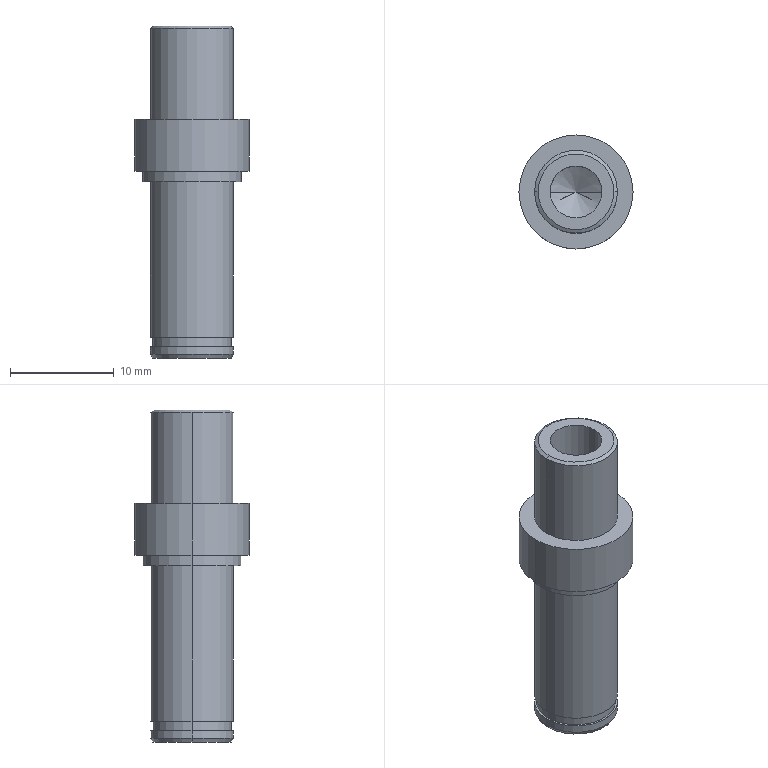Part | STEP file | FBDS-CS-032 | 1 solid | 27 faces | box 11 x 11 x 32 mm | volume 1542 mm3 | cylinder 14 | plane 7 | cone 6 | commonest cylinder face diameters 8 x6 5 x2 7.6 x2 9.5 x2 11 x2
STEP:
#1=CARTESIAN_POINT('',(3.654,0.,32.));
#2=VERTEX_POINT('',#1);
#3=CARTESIAN_POINT('',(-3.654,0.,32.));
#4=VERTEX_POINT('',#3);
#5=CARTESIAN_POINT('',(0.,0.,32.));
#6=DIRECTION('',(0.,0.,1.));
#7=DIRECTION('',(1.,0.,0.));
#8=AXIS2_PLACEMENT_3D('',#5,#6,#7);
#9=CIRCLE('',#8,3.654);
#10=EDGE_CURVE('',#2,#4,#9,.T.);
#11=ORIENTED_EDGE('',*,*,#10,.F.);
#12=CARTESIAN_POINT('',(4.,0.,31.8));
#13=VERTEX_POINT('',#12);
#14=CARTESIAN_POINT('',(3.654,0.,32.));
#15=DIRECTION('',(0.866,0.,-0.5));
#16=VECTOR('',#15,1000.);
#17=LINE('',#14,#16);
#18=EDGE_CURVE('',#2,#13,#17,.T.);
#19=ORIENTED_EDGE('',*,*,#18,.T.);
#20=CARTESIAN_POINT('',(-4.,0.,31.8));
#21=VERTEX_POINT('',#20);
#22=CARTESIAN_POINT('',(0.,0.,31.8));
#23=DIRECTION('',(0.,0.,-1.));
#24=DIRECTION('',(1.,0.,0.));
#25=AXIS2_PLACEMENT_3D('',#22,#23,#24);
#26=CIRCLE('',#25,4.);
#27=EDGE_CURVE('',#21,#13,#26,.T.);
#28=ORIENTED_EDGE('',*,*,#27,.F.);
#29=CARTESIAN_POINT('',(-3.654,0.,32.));
#30=DIRECTION('',(-0.866,0.,-0.5));
#31=VECTOR('',#30,1000.);
#32=LINE('',#29,#31);
#33=EDGE_CURVE('',#4,#21,#32,.T.);
#34=ORIENTED_EDGE('',*,*,#33,.F.);
#35=EDGE_LOOP('',(#11,#19,#28,#34));
#36=FACE_OUTER_BOUND('',#35,.T.);
#37=CARTESIAN_POINT('',(0.,0.,32.));
#38=DIRECTION('',(0.,0.,-1.));
#39=DIRECTION('',(-1.,0.,0.));
#40=AXIS2_PLACEMENT_3D('',#37,#38,#39);
#41=CONICAL_SURFACE('',#40,3.654,1.047);
#42=ADVANCED_FACE('',(#36),#41,.T.);
#43=CARTESIAN_POINT('',(-3.8,0.,0.));
#44=VERTEX_POINT('',#43);
#45=CARTESIAN_POINT('',(3.8,0.,0.));
#46=VERTEX_POINT('',#45);
#47=CARTESIAN_POINT('',(0.,0.,0.));
#48=DIRECTION('',(0.,0.,-1.));
#49=DIRECTION('',(1.,0.,0.));
#50=AXIS2_PLACEMENT_3D('',#47,#48,#49);
#51=CIRCLE('',#50,3.8);
#52=EDGE_CURVE('',#44,#46,#51,.T.);
#53=ORIENTED_EDGE('',*,*,#52,.F.);
#54=CARTESIAN_POINT('',(-4.,0.,0.3464));
#55=VERTEX_POINT('',#54);
#56=CARTESIAN_POINT('',(-4.,0.,0.3464));
#57=DIRECTION('',(-0.5,0.,0.866));
#58=VECTOR('',#57,1000.);
#59=LINE('',#56,#58);
#60=EDGE_CURVE('',#44,#55,#59,.T.);
#61=ORIENTED_EDGE('',*,*,#60,.T.);
#62=CARTESIAN_POINT('',(4.,0.,0.3464));
#63=VERTEX_POINT('',#62);
#64=CARTESIAN_POINT('',(0.,0.,0.3464));
#65=DIRECTION('',(0.,0.,1.));
#66=DIRECTION('',(1.,0.,0.));
#67=AXIS2_PLACEMENT_3D('',#64,#65,#66);
#68=CIRCLE('',#67,4.);
#69=EDGE_CURVE('',#63,#55,#68,.T.);
#70=ORIENTED_EDGE('',*,*,#69,.F.);
#71=CARTESIAN_POINT('',(4.,0.,0.3464));
#72=DIRECTION('',(0.5,0.,0.866));
#73=VECTOR('',#72,1000.);
#74=LINE('',#71,#73);
#75=EDGE_CURVE('',#46,#63,#74,.T.);
#76=ORIENTED_EDGE('',*,*,#75,.F.);
#77=EDGE_LOOP('',(#53,#61,#70,#76));
#78=FACE_OUTER_BOUND('',#77,.T.);
#79=CARTESIAN_POINT('',(0.,0.,0.3464));
#80=DIRECTION('',(0.,0.,1.));
#81=DIRECTION('',(1.,0.,0.));
#82=AXIS2_PLACEMENT_3D('',#79,#80,#81);
#83=CONICAL_SURFACE('',#82,4.,0.5236);
#84=ADVANCED_FACE('',(#78),#83,.T.);
#85=CARTESIAN_POINT('',(-2.5,0.,17.));
#86=VERTEX_POINT('',#85);
#87=CARTESIAN_POINT('',(2.5,0.,17.));
#88=VERTEX_POINT('',#87);
#89=CARTESIAN_POINT('',(0.,0.,17.));
#90=DIRECTION('',(0.,0.,1.));
#91=DIRECTION('',(1.,0.,0.));
#92=AXIS2_PLACEMENT_3D('',#89,#90,#91);
#93=CIRCLE('',#92,2.5);
#94=EDGE_CURVE('',#86,#88,#93,.T.);
#95=ORIENTED_EDGE('',*,*,#94,.F.);
#96=CARTESIAN_POINT('',(-2.5,0.,32.));
#97=VERTEX_POINT('',#96);
#98=CARTESIAN_POINT('',(-2.5,0.,32.));
#99=DIRECTION('',(0.,0.,1.));
#100=VECTOR('',#99,1000.);
#101=LINE('',#98,#100);
#102=EDGE_CURVE('',#86,#97,#101,.T.);
#103=ORIENTED_EDGE('',*,*,#102,.T.);
#104=CARTESIAN_POINT('',(2.5,0.,32.));
#105=VERTEX_POINT('',#104);
#106=CARTESIAN_POINT('',(0.,0.,32.));
#107=DIRECTION('',(0.,0.,1.));
#108=DIRECTION('',(1.,0.,0.));
#109=AXIS2_PLACEMENT_3D('',#106,#107,#108);
#110=CIRCLE('',#109,2.5);
#111=EDGE_CURVE('',#97,#105,#110,.T.);
#112=ORIENTED_EDGE('',*,*,#111,.T.);
#113=CARTESIAN_POINT('',(2.5,0.,32.));
#114=DIRECTION('',(0.,0.,1.));
#115=VECTOR('',#114,1000.);
#116=LINE('',#113,#115);
#117=EDGE_CURVE('',#88,#105,#116,.T.);
#118=ORIENTED_EDGE('',*,*,#117,.F.);
#119=EDGE_LOOP('',(#95,#103,#112,#118));
#120=FACE_OUTER_BOUND('',#119,.T.);
#121=CARTESIAN_POINT('',(0.,0.,32.));
#122=DIRECTION('',(0.,0.,1.));
#123=DIRECTION('',(1.,0.,0.));
#124=AXIS2_PLACEMENT_3D('',#121,#122,#123);
#125=CYLINDRICAL_SURFACE('',#124,2.5);
#126=ADVANCED_FACE('',(#120),#125,.F.);
#127=CARTESIAN_POINT('',(0.,0.,15.498));
#128=VERTEX_POINT('',#127);
#129=CARTESIAN_POINT('',(2.5,0.,17.));
#130=DIRECTION('',(0.8572,0.,0.515));
#131=VECTOR('',#130,1000.);
#132=LINE('',#129,#131);
#133=EDGE_CURVE('',#128,#88,#132,.T.);
#134=ORIENTED_EDGE('',*,*,#133,.F.);
#135=CARTESIAN_POINT('',(-2.5,0.,17.));
#136=DIRECTION('',(-0.8572,0.,0.515));
#137=VECTOR('',#136,1000.);
#138=LINE('',#135,#137);
#139=EDGE_CURVE('',#128,#86,#138,.T.);
#140=ORIENTED_EDGE('',*,*,#139,.T.);
#141=ORIENTED_EDGE('',*,*,#94,.T.);
#142=EDGE_LOOP('',(#134,#140,#141));
#143=FACE_OUTER_BOUND('',#142,.T.);
#144=CARTESIAN_POINT('',(0.,0.,17.));
#145=DIRECTION('',(0.,0.,1.));
#146=DIRECTION('',(1.,0.,0.));
#147=AXIS2_PLACEMENT_3D('',#144,#145,#146);
#148=CONICAL_SURFACE('',#147,2.5,1.03);
#149=ADVANCED_FACE('',(#143),#148,.F.);
#150=ORIENTED_EDGE('',*,*,#27,.T.);
#151=CARTESIAN_POINT('',(4.,0.,23.));
#152=VERTEX_POINT('',#151);
#153=CARTESIAN_POINT('',(4.,0.,32.));
#154=DIRECTION('',(0.,0.,-1.));
#155=VECTOR('',#154,1000.);
#156=LINE('',#153,#155);
#157=EDGE_CURVE('',#13,#152,#156,.T.);
#158=ORIENTED_EDGE('',*,*,#157,.T.);
#159=CARTESIAN_POINT('',(-4.,0.,23.));
#160=VERTEX_POINT('',#159);
#161=CARTESIAN_POINT('',(0.,0.,23.));
#162=DIRECTION('',(0.,0.,1.));
#163=DIRECTION('',(1.,0.,0.));
#164=AXIS2_PLACEMENT_3D('',#161,#162,#163);
#165=CIRCLE('',#164,4.);
#166=EDGE_CURVE('',#152,#160,#165,.T.);
#167=ORIENTED_EDGE('',*,*,#166,.T.);
#168=CARTESIAN_POINT('',(-4.,0.,32.));
#169=DIRECTION('',(0.,0.,-1.));
#170=VECTOR('',#169,1000.);
#171=LINE('',#168,#170);
#172=EDGE_CURVE('',#21,#160,#171,.T.);
#173=ORIENTED_EDGE('',*,*,#172,.F.);
#174=EDGE_LOOP('',(#150,#158,#167,#173));
#175=FACE_OUTER_BOUND('',#174,.T.);
#176=CARTESIAN_POINT('',(0.,0.,32.));
#177=DIRECTION('',(0.,0.,-1.));
#178=DIRECTION('',(-1.,0.,0.));
#179=AXIS2_PLACEMENT_3D('',#176,#177,#178);
#180=CYLINDRICAL_SURFACE('',#179,4.);
#181=ADVANCED_FACE('',(#175),#180,.T.);
#182=CARTESIAN_POINT('',(-4.,0.,1.1));
#183=VERTEX_POINT('',#182);
#184=CARTESIAN_POINT('',(4.,0.,1.1));
#185=VERTEX_POINT('',#184);
#186=CARTESIAN_POINT('',(0.,0.,1.1));
#187=DIRECTION('',(0.,0.,-1.));
#188=DIRECTION('',(-1.,0.,0.));
#189=AXIS2_PLACEMENT_3D('',#186,#187,#188);
#190=CIRCLE('',#189,4.);
#191=EDGE_CURVE('',#183,#185,#190,.T.);
#192=ORIENTED_EDGE('',*,*,#191,.T.);
#193=CARTESIAN_POINT('',(4.,0.,17.));
#194=DIRECTION('',(0.,0.,-1.));
#195=VECTOR('',#194,1000.);
#196=LINE('',#193,#195);
#197=EDGE_CURVE('',#185,#63,#196,.T.);
#198=ORIENTED_EDGE('',*,*,#197,.T.);
#199=ORIENTED_EDGE('',*,*,#69,.T.);
#200=CARTESIAN_POINT('',(-4.,0.,17.));
#201=DIRECTION('',(0.,0.,-1.));
#202=VECTOR('',#201,1000.);
#203=LINE('',#200,#202);
#204=EDGE_CURVE('',#183,#55,#203,.T.);
#205=ORIENTED_EDGE('',*,*,#204,.F.);
#206=EDGE_LOOP('',(#192,#198,#199,#205));
#207=FACE_OUTER_BOUND('',#206,.T.);
#208=CARTESIAN_POINT('',(0.,0.,17.));
#209=DIRECTION('',(0.,0.,-1.));
#210=DIRECTION('',(-1.,0.,0.));
#211=AXIS2_PLACEMENT_3D('',#208,#209,#210);
#212=CYLINDRICAL_SURFACE('',#211,4.);
#213=ADVANCED_FACE('',(#207),#212,.T.);
#214=CARTESIAN_POINT('',(-3.8,0.,1.1));
#215=VERTEX_POINT('',#214);
#216=CARTESIAN_POINT('',(3.8,0.,1.1));
#217=VERTEX_POINT('',#216);
#218=CARTESIAN_POINT('',(0.,0.,1.1));
#219=DIRECTION('',(0.,0.,-1.));
#220=DIRECTION('',(-1.,0.,0.));
#221=AXIS2_PLACEMENT_3D('',#218,#219,#220);
#222=CIRCLE('',#221,3.8);
#223=EDGE_CURVE('',#215,#217,#222,.T.);
#224=ORIENTED_EDGE('',*,*,#223,.F.);
#225=CARTESIAN_POINT('',(-3.8,0.,2.));
#226=VERTEX_POINT('',#225);
#227=CARTESIAN_POINT('',(-3.8,0.,1.1));
#228=DIRECTION('',(0.,0.,1.));
#229=VECTOR('',#228,1000.);
#230=LINE('',#227,#229);
#231=EDGE_CURVE('',#215,#226,#230,.T.);
#232=ORIENTED_EDGE('',*,*,#231,.T.);
#233=CARTESIAN_POINT('',(3.8,0.,2.));
#234=VERTEX_POINT('',#233);
#235=CARTESIAN_POINT('',(0.,0.,2.));
#236=DIRECTION('',(0.,0.,-1.));
#237=DIRECTION('',(-1.,0.,0.));
#238=AXIS2_PLACEMENT_3D('',#235,#236,#237);
#239=CIRCLE('',#238,3.8);
#240=EDGE_CURVE('',#226,#234,#239,.T.);
#241=ORIENTED_EDGE('',*,*,#240,.T.);
#242=CARTESIAN_POINT('',(3.8,0.,1.1));
#243=DIRECTION('',(0.,0.,1.));
#244=VECTOR('',#243,1000.);
#245=LINE('',#242,#244);
#246=EDGE_CURVE('',#217,#234,#245,.T.);
#247=ORIENTED_EDGE('',*,*,#246,.F.);
#248=EDGE_LOOP('',(#224,#232,#241,#247));
#249=FACE_OUTER_BOUND('',#248,.T.);
#250=CARTESIAN_POINT('',(0.,0.,1.1));
#251=DIRECTION('',(0.,0.,1.));
#252=DIRECTION('',(1.,0.,0.));
#253=AXIS2_PLACEMENT_3D('',#250,#251,#252);
#254=CYLINDRICAL_SURFACE('',#253,3.8);
#255=ADVANCED_FACE('',(#249),#254,.T.);
#256=CARTESIAN_POINT('',(5.5,0.,23.));
#257=VERTEX_POINT('',#256);
#258=CARTESIAN_POINT('',(-5.5,0.,23.));
#259=VERTEX_POINT('',#258);
#260=CARTESIAN_POINT('',(0.,0.,23.));
#261=DIRECTION('',(0.,0.,1.));
#262=DIRECTION('',(1.,0.,0.));
#263=AXIS2_PLACEMENT_3D('',#260,#261,#262);
#264=CIRCLE('',#263,5.5);
#265=EDGE_CURVE('',#257,#259,#264,.T.);
#266=ORIENTED_EDGE('',*,*,#265,.F.);
#267=CARTESIAN_POINT('',(5.5,0.,18.));
#268=VERTEX_POINT('',#267);
#269=CARTESIAN_POINT('',(5.5,0.,23.));
#270=DIRECTION('',(0.,0.,-1.));
#271=VECTOR('',#270,1000.);
#272=LINE('',#269,#271);
#273=EDGE_CURVE('',#257,#268,#272,.T.);
#274=ORIENTED_EDGE('',*,*,#273,.T.);
#275=CARTESIAN_POINT('',(-5.5,0.,18.));
#276=VERTEX_POINT('',#275);
#277=CARTESIAN_POINT('',(0.,0.,18.));
#278=DIRECTION('',(0.,0.,1.));
#279=DIRECTION('',(1.,0.,0.));
#280=AXIS2_PLACEMENT_3D('',#277,#278,#279);
#281=CIRCLE('',#280,5.5);
#282=EDGE_CURVE('',#268,#276,#281,.T.);
#283=ORIENTED_EDGE('',*,*,#282,.T.);
#284=CARTESIAN_POINT('',(-5.5,0.,23.));
#285=DIRECTION('',(0.,0.,-1.));
#286=VECTOR('',#285,1000.);
#287=LINE('',#284,#286);
#288=EDGE_CURVE('',#259,#276,#287,.T.);
#289=ORIENTED_EDGE('',*,*,#288,.F.);
#290=EDGE_LOOP('',(#266,#274,#283,#289));
#291=FACE_OUTER_BOUND('',#290,.T.);
#292=CARTESIAN_POINT('',(0.,0.,23.));
#293=DIRECTION('',(0.,0.,-1.));
#294=DIRECTION('',(-1.,0.,0.));
#295=AXIS2_PLACEMENT_3D('',#292,#293,#294);
#296=CYLINDRICAL_SURFACE('',#295,5.5);
#297=ADVANCED_FACE('',(#291),#296,.T.);
#298=CARTESIAN_POINT('',(4.75,0.,18.));
#299=VERTEX_POINT('',#298);
#300=CARTESIAN_POINT('',(-4.75,0.,18.));
#301=VERTEX_POINT('',#300);
#302=CARTESIAN_POINT('',(0.,0.,18.));
#303=DIRECTION('',(0.,0.,1.));
#304=DIRECTION('',(1.,0.,0.));
#305=AXIS2_PLACEMENT_3D('',#302,#303,#304);
#306=CIRCLE('',#305,4.75);
#307=EDGE_CURVE('',#299,#301,#306,.T.);
#308=ORIENTED_EDGE('',*,*,#307,.F.);
#309=CARTESIAN_POINT('',(4.75,0.,17.));
#310=VERTEX_POINT('',#309);
#311=CARTESIAN_POINT('',(4.75,0.,18.));
#312=DIRECTION('',(0.,0.,-1.));
#313=VECTOR('',#312,1000.);
#314=LINE('',#311,#313);
#315=EDGE_CURVE('',#299,#310,#314,.T.);
#316=ORIENTED_EDGE('',*,*,#315,.T.);
#317=CARTESIAN_POINT('',(-4.75,0.,17.));
#318=VERTEX_POINT('',#317);
#319=CARTESIAN_POINT('',(0.,0.,17.));
#320=DIRECTION('',(0.,0.,1.));
#321=DIRECTION('',(1.,0.,0.));
#322=AXIS2_PLACEMENT_3D('',#319,#320,#321);
#323=CIRCLE('',#322,4.75);
#324=EDGE_CURVE('',#310,#318,#323,.T.);
#325=ORIENTED_EDGE('',*,*,#324,.T.);
#326=CARTESIAN_POINT('',(-4.75,0.,18.));
#327=DIRECTION('',(0.,0.,-1.));
#328=VECTOR('',#327,1000.);
#329=LINE('',#326,#328);
#330=EDGE_CURVE('',#301,#318,#329,.T.);
#331=ORIENTED_EDGE('',*,*,#330,.F.);
#332=EDGE_LOOP('',(#308,#316,#325,#331));
#333=FACE_OUTER_BOUND('',#332,.T.);
#334=CARTESIAN_POINT('',(0.,0.,18.));
#335=DIRECTION('',(0.,0.,-1.));
#336=DIRECTION('',(-1.,0.,0.));
#337=AXIS2_PLACEMENT_3D('',#334,#335,#336);
#338=CYLINDRICAL_SURFACE('',#337,4.75);
#339=ADVANCED_FACE('',(#333),#338,.T.);
#340=CARTESIAN_POINT('',(4.,0.,17.));
#341=VERTEX_POINT('',#340);
#342=CARTESIAN_POINT('',(-4.,0.,17.));
#343=VERTEX_POINT('',#342);
#344=CARTESIAN_POINT('',(0.,0.,17.));
#345=DIRECTION('',(0.,0.,1.));
#346=DIRECTION('',(1.,0.,0.));
#347=AXIS2_PLACEMENT_3D('',#344,#345,#346);
#348=CIRCLE('',#347,4.);
#349=EDGE_CURVE('',#341,#343,#348,.T.);
#350=ORIENTED_EDGE('',*,*,#349,.F.);
#351=CARTESIAN_POINT('',(4.,0.,2.));
#352=VERTEX_POINT('',#351);
#353=CARTESIAN_POINT('',(4.,0.,17.));
#354=DIRECTION('',(0.,0.,-1.));
#355=VECTOR('',#354,1000.);
#356=LINE('',#353,#355);
#357=EDGE_CURVE('',#341,#352,#356,.T.);
#358=ORIENTED_EDGE('',*,*,#357,.T.);
#359=CARTESIAN_POINT('',(-4.,0.,2.));
#360=VERTEX_POINT('',#359);
#361=CARTESIAN_POINT('',(0.,0.,2.));
#362=DIRECTION('',(0.,0.,-1.));
#363=DIRECTION('',(-1.,0.,0.));
#364=AXIS2_PLACEMENT_3D('',#361,#362,#363);
#365=CIRCLE('',#364,4.);
#366=EDGE_CURVE('',#360,#352,#365,.T.);
#367=ORIENTED_EDGE('',*,*,#366,.F.);
#368=CARTESIAN_POINT('',(-4.,0.,17.));
#369=DIRECTION('',(0.,0.,-1.));
#370=VECTOR('',#369,1000.);
#371=LINE('',#368,#370);
#372=EDGE_CURVE('',#343,#360,#371,.T.);
#373=ORIENTED_EDGE('',*,*,#372,.F.);
#374=EDGE_LOOP('',(#350,#358,#367,#373));
#375=FACE_OUTER_BOUND('',#374,.T.);
#376=CARTESIAN_POINT('',(0.,0.,17.));
#377=DIRECTION('',(0.,0.,-1.));
#378=DIRECTION('',(-1.,0.,0.));
#379=AXIS2_PLACEMENT_3D('',#376,#377,#378);
#380=CYLINDRICAL_SURFACE('',#379,4.);
#381=ADVANCED_FACE('',(#375),#380,.T.);
#382=ORIENTED_EDGE('',*,*,#357,.F.);
#383=CARTESIAN_POINT('',(0.,0.,17.));
#384=DIRECTION('',(0.,0.,1.));
#385=DIRECTION('',(1.,0.,0.));
#386=AXIS2_PLACEMENT_3D('',#383,#384,#385);
#387=CIRCLE('',#386,4.);
#388=EDGE_CURVE('',#343,#341,#387,.T.);
#389=ORIENTED_EDGE('',*,*,#388,.F.);
#390=ORIENTED_EDGE('',*,*,#372,.T.);
#391=CARTESIAN_POINT('',(0.,0.,2.));
#392=DIRECTION('',(0.,0.,-1.));
#393=DIRECTION('',(-1.,0.,0.));
#394=AXIS2_PLACEMENT_3D('',#391,#392,#393);
#395=CIRCLE('',#394,4.);
#396=EDGE_CURVE('',#352,#360,#395,.T.);
#397=ORIENTED_EDGE('',*,*,#396,.F.);
#398=EDGE_LOOP('',(#382,#389,#390,#397));
#399=FACE_OUTER_BOUND('',#398,.T.);
#400=CARTESIAN_POINT('',(0.,0.,17.));
#401=DIRECTION('',(0.,0.,-1.));
#402=DIRECTION('',(-1.,0.,0.));
#403=AXIS2_PLACEMENT_3D('',#400,#401,#402);
#404=CYLINDRICAL_SURFACE('',#403,4.);
#405=ADVANCED_FACE('',(#399),#404,.T.);
#406=ORIENTED_EDGE('',*,*,#315,.F.);
#407=CARTESIAN_POINT('',(0.,0.,18.));
#408=DIRECTION('',(0.,0.,1.));
#409=DIRECTION('',(1.,0.,0.));
#410=AXIS2_PLACEMENT_3D('',#407,#408,#409);
#411=CIRCLE('',#410,4.75);
#412=EDGE_CURVE('',#301,#299,#411,.T.);
#413=ORIENTED_EDGE('',*,*,#412,.F.);
#414=ORIENTED_EDGE('',*,*,#330,.T.);
#415=CARTESIAN_POINT('',(0.,0.,17.));
#416=DIRECTION('',(0.,0.,1.));
#417=DIRECTION('',(1.,0.,0.));
#418=AXIS2_PLACEMENT_3D('',#415,#416,#417);
#419=CIRCLE('',#418,4.75);
#420=EDGE_CURVE('',#318,#310,#419,.T.);
#421=ORIENTED_EDGE('',*,*,#420,.T.);
#422=EDGE_LOOP('',(#406,#413,#414,#421));
#423=FACE_OUTER_BOUND('',#422,.T.);
#424=CARTESIAN_POINT('',(0.,0.,18.));
#425=DIRECTION('',(0.,0.,-1.));
#426=DIRECTION('',(-1.,0.,0.));
#427=AXIS2_PLACEMENT_3D('',#424,#425,#426);
#428=CYLINDRICAL_SURFACE('',#427,4.75);
#429=ADVANCED_FACE('',(#423),#428,.T.);
#430=ORIENTED_EDGE('',*,*,#388,.T.);
#431=ORIENTED_EDGE('',*,*,#349,.T.);
#432=EDGE_LOOP('',(#430,#431));
#433=FACE_BOUND('',#432,.T.);
#434=ORIENTED_EDGE('',*,*,#420,.F.);
#435=ORIENTED_EDGE('',*,*,#324,.F.);
#436=EDGE_LOOP('',(#434,#435));
#437=FACE_OUTER_BOUND('',#436,.T.);
#438=CARTESIAN_POINT('',(0.,0.,17.));
#439=DIRECTION('',(0.,0.,1.));
#440=DIRECTION('',(1.,0.,0.));
#441=AXIS2_PLACEMENT_3D('',#438,#439,#440);
#442=PLANE('',#441);
#443=ADVANCED_FACE('',(#433,#437),#442,.F.);
#444=ORIENTED_EDGE('',*,*,#273,.F.);
#445=CARTESIAN_POINT('',(0.,0.,23.));
#446=DIRECTION('',(0.,0.,1.));
#447=DIRECTION('',(1.,0.,0.));
#448=AXIS2_PLACEMENT_3D('',#445,#446,#447);
#449=CIRCLE('',#448,5.5);
#450=EDGE_CURVE('',#259,#257,#449,.T.);
#451=ORIENTED_EDGE('',*,*,#450,.F.);
#452=ORIENTED_EDGE('',*,*,#288,.T.);
#453=CARTESIAN_POINT('',(0.,0.,18.));
#454=DIRECTION('',(0.,0.,1.));
#455=DIRECTION('',(1.,0.,0.));
#456=AXIS2_PLACEMENT_3D('',#453,#454,#455);
#457=CIRCLE('',#456,5.5);
#458=EDGE_CURVE('',#276,#268,#457,.T.);
#459=ORIENTED_EDGE('',*,*,#458,.T.);
#460=EDGE_LOOP('',(#444,#451,#452,#459));
#461=FACE_OUTER_BOUND('',#460,.T.);
#462=CARTESIAN_POINT('',(0.,0.,23.));
#463=DIRECTION('',(0.,0.,-1.));
#464=DIRECTION('',(-1.,0.,0.));
#465=AXIS2_PLACEMENT_3D('',#462,#463,#464);
#466=CYLINDRICAL_SURFACE('',#465,5.5);
#467=ADVANCED_FACE('',(#461),#466,.T.);
#468=CARTESIAN_POINT('',(0.,0.,23.));
#469=DIRECTION('',(0.,0.,1.));
#470=DIRECTION('',(1.,0.,0.));
#471=AXIS2_PLACEMENT_3D('',#468,#469,#470);
#472=CIRCLE('',#471,4.);
#473=EDGE_CURVE('',#160,#152,#472,.T.);
#474=ORIENTED_EDGE('',*,*,#473,.F.);
#475=ORIENTED_EDGE('',*,*,#166,.F.);
#476=EDGE_LOOP('',(#474,#475));
#477=FACE_BOUND('',#476,.T.);
#478=ORIENTED_EDGE('',*,*,#450,.T.);
#479=ORIENTED_EDGE('',*,*,#265,.T.);
#480=EDGE_LOOP('',(#478,#479));
#481=FACE_OUTER_BOUND('',#480,.T.);
#482=CARTESIAN_POINT('',(0.,0.,23.));
#483=DIRECTION('',(0.,0.,1.));
#484=DIRECTION('',(1.,0.,0.));
#485=AXIS2_PLACEMENT_3D('',#482,#483,#484);
#486=PLANE('',#485);
#487=ADVANCED_FACE('',(#477,#481),#486,.T.);
#488=ORIENTED_EDGE('',*,*,#412,.T.);
#489=ORIENTED_EDGE('',*,*,#307,.T.);
#490=EDGE_LOOP('',(#488,#489));
#491=FACE_BOUND('',#490,.T.);
#492=ORIENTED_EDGE('',*,*,#458,.F.);
#493=ORIENTED_EDGE('',*,*,#282,.F.);
#494=EDGE_LOOP('',(#492,#493));
#495=FACE_OUTER_BOUND('',#494,.T.);
#496=CARTESIAN_POINT('',(0.,0.,18.));
#497=DIRECTION('',(0.,0.,1.));
#498=DIRECTION('',(1.,0.,0.));
#499=AXIS2_PLACEMENT_3D('',#496,#497,#498);
#500=PLANE('',#499);
#501=ADVANCED_FACE('',(#491,#495),#500,.F.);
#502=CARTESIAN_POINT('',(0.,0.,1.1));
#503=DIRECTION('',(0.,0.,-1.));
#504=DIRECTION('',(-1.,0.,0.));
#505=AXIS2_PLACEMENT_3D('',#502,#503,#504);
#506=CIRCLE('',#505,3.8);
#507=EDGE_CURVE('',#217,#215,#506,.T.);
#508=ORIENTED_EDGE('',*,*,#507,.T.);
#509=ORIENTED_EDGE('',*,*,#223,.T.);
#510=EDGE_LOOP('',(#508,#509));
#511=FACE_BOUND('',#510,.T.);
#512=ORIENTED_EDGE('',*,*,#191,.F.);
#513=CARTESIAN_POINT('',(0.,0.,1.1));
#514=DIRECTION('',(0.,0.,-1.));
#515=DIRECTION('',(-1.,0.,0.));
#516=AXIS2_PLACEMENT_3D('',#513,#514,#515);
#517=CIRCLE('',#516,4.);
#518=EDGE_CURVE('',#185,#183,#517,.T.);
#519=ORIENTED_EDGE('',*,*,#518,.F.);
#520=EDGE_LOOP('',(#512,#519));
#521=FACE_OUTER_BOUND('',#520,.T.);
#522=CARTESIAN_POINT('',(0.,0.,1.1));
#523=DIRECTION('',(0.,0.,-1.));
#524=DIRECTION('',(-1.,0.,0.));
#525=AXIS2_PLACEMENT_3D('',#522,#523,#524);
#526=PLANE('',#525);
#527=ADVANCED_FACE('',(#511,#521),#526,.F.);
#528=CARTESIAN_POINT('',(0.,0.,2.));
#529=DIRECTION('',(0.,0.,-1.));
#530=DIRECTION('',(-1.,0.,0.));
#531=AXIS2_PLACEMENT_3D('',#528,#529,#530);
#532=CIRCLE('',#531,3.8);
#533=EDGE_CURVE('',#234,#226,#532,.T.);
#534=ORIENTED_EDGE('',*,*,#533,.F.);
#535=ORIENTED_EDGE('',*,*,#240,.F.);
#536=EDGE_LOOP('',(#534,#535));
#537=FACE_BOUND('',#536,.T.);
#538=ORIENTED_EDGE('',*,*,#366,.T.);
#539=ORIENTED_EDGE('',*,*,#396,.T.);
#540=EDGE_LOOP('',(#538,#539));
#541=FACE_OUTER_BOUND('',#540,.T.);
#542=CARTESIAN_POINT('',(0.,0.,2.));
#543=DIRECTION('',(0.,0.,-1.));
#544=DIRECTION('',(-1.,0.,0.));
#545=AXIS2_PLACEMENT_3D('',#542,#543,#544);
#546=PLANE('',#545);
#547=ADVANCED_FACE('',(#537,#541),#546,.T.);
#548=ORIENTED_EDGE('',*,*,#231,.F.);
#549=ORIENTED_EDGE('',*,*,#507,.F.);
#550=ORIENTED_EDGE('',*,*,#246,.T.);
#551=ORIENTED_EDGE('',*,*,#533,.T.);
#552=EDGE_LOOP('',(#548,#549,#550,#551));
#553=FACE_OUTER_BOUND('',#552,.T.);
#554=CARTESIAN_POINT('',(0.,0.,1.1));
#555=DIRECTION('',(0.,0.,1.));
#556=DIRECTION('',(1.,0.,0.));
#557=AXIS2_PLACEMENT_3D('',#554,#555,#556);
#558=CYLINDRICAL_SURFACE('',#557,3.8);
#559=ADVANCED_FACE('',(#553),#558,.T.);
#560=CARTESIAN_POINT('',(0.,0.,0.));
#561=DIRECTION('',(0.,0.,-1.));
#562=DIRECTION('',(1.,0.,0.));
#563=AXIS2_PLACEMENT_3D('',#560,#561,#562);
#564=CIRCLE('',#563,3.8);
#565=EDGE_CURVE('',#46,#44,#564,.T.);
#566=ORIENTED_EDGE('',*,*,#565,.T.);
#567=ORIENTED_EDGE('',*,*,#52,.T.);
#568=EDGE_LOOP('',(#566,#567));
#569=FACE_OUTER_BOUND('',#568,.T.);
#570=CARTESIAN_POINT('',(0.,0.,0.));
#571=DIRECTION('',(0.,0.,1.));
#572=DIRECTION('',(1.,0.,0.));
#573=AXIS2_PLACEMENT_3D('',#570,#571,#572);
#574=PLANE('',#573);
#575=ADVANCED_FACE('',(#569),#574,.F.);
#576=ORIENTED_EDGE('',*,*,#197,.F.);
#577=ORIENTED_EDGE('',*,*,#518,.T.);
#578=ORIENTED_EDGE('',*,*,#204,.T.);
#579=CARTESIAN_POINT('',(0.,0.,0.3464));
#580=DIRECTION('',(0.,0.,1.));
#581=DIRECTION('',(1.,0.,0.));
#582=AXIS2_PLACEMENT_3D('',#579,#580,#581);
#583=CIRCLE('',#582,4.);
#584=EDGE_CURVE('',#55,#63,#583,.T.);
#585=ORIENTED_EDGE('',*,*,#584,.T.);
#586=EDGE_LOOP('',(#576,#577,#578,#585));
#587=FACE_OUTER_BOUND('',#586,.T.);
#588=CARTESIAN_POINT('',(0.,0.,17.));
#589=DIRECTION('',(0.,0.,-1.));
#590=DIRECTION('',(-1.,0.,0.));
#591=AXIS2_PLACEMENT_3D('',#588,#589,#590);
#592=CYLINDRICAL_SURFACE('',#591,4.);
#593=ADVANCED_FACE('',(#587),#592,.T.);
#594=ORIENTED_EDGE('',*,*,#157,.F.);
#595=CARTESIAN_POINT('',(0.,0.,31.8));
#596=DIRECTION('',(0.,0.,-1.));
#597=DIRECTION('',(1.,0.,0.));
#598=AXIS2_PLACEMENT_3D('',#595,#596,#597);
#599=CIRCLE('',#598,4.);
#600=EDGE_CURVE('',#13,#21,#599,.T.);
#601=ORIENTED_EDGE('',*,*,#600,.T.);
#602=ORIENTED_EDGE('',*,*,#172,.T.);
#603=ORIENTED_EDGE('',*,*,#473,.T.);
#604=EDGE_LOOP('',(#594,#601,#602,#603));
#605=FACE_OUTER_BOUND('',#604,.T.);
#606=CARTESIAN_POINT('',(0.,0.,32.));
#607=DIRECTION('',(0.,0.,-1.));
#608=DIRECTION('',(-1.,0.,0.));
#609=AXIS2_PLACEMENT_3D('',#606,#607,#608);
#610=CYLINDRICAL_SURFACE('',#609,4.);
#611=ADVANCED_FACE('',(#605),#610,.T.);
#612=CARTESIAN_POINT('',(0.,0.,32.));
#613=DIRECTION('',(0.,0.,1.));
#614=DIRECTION('',(1.,0.,0.));
#615=AXIS2_PLACEMENT_3D('',#612,#613,#614);
#616=CIRCLE('',#615,3.654);
#617=EDGE_CURVE('',#4,#2,#616,.T.);
#618=ORIENTED_EDGE('',*,*,#617,.T.);
#619=ORIENTED_EDGE('',*,*,#10,.T.);
#620=EDGE_LOOP('',(#618,#619));
#621=FACE_OUTER_BOUND('',#620,.T.);
#622=CARTESIAN_POINT('',(0.,0.,32.));
#623=DIRECTION('',(0.,0.,1.));
#624=DIRECTION('',(1.,0.,0.));
#625=AXIS2_PLACEMENT_3D('',#622,#623,#624);
#626=CIRCLE('',#625,2.5);
#627=EDGE_CURVE('',#105,#97,#626,.T.);
#628=ORIENTED_EDGE('',*,*,#627,.F.);
#629=ORIENTED_EDGE('',*,*,#111,.F.);
#630=EDGE_LOOP('',(#628,#629));
#631=FACE_BOUND('',#630,.T.);
#632=CARTESIAN_POINT('',(0.,0.,32.));
#633=DIRECTION('',(0.,0.,1.));
#634=DIRECTION('',(1.,0.,0.));
#635=AXIS2_PLACEMENT_3D('',#632,#633,#634);
#636=PLANE('',#635);
#637=ADVANCED_FACE('',(#621,#631),#636,.T.);
#638=ORIENTED_EDGE('',*,*,#139,.F.);
#639=ORIENTED_EDGE('',*,*,#133,.T.);
#640=CARTESIAN_POINT('',(0.,0.,17.));
#641=DIRECTION('',(0.,0.,1.));
#642=DIRECTION('',(1.,0.,0.));
#643=AXIS2_PLACEMENT_3D('',#640,#641,#642);
#644=CIRCLE('',#643,2.5);
#645=EDGE_CURVE('',#88,#86,#644,.T.);
#646=ORIENTED_EDGE('',*,*,#645,.T.);
#647=EDGE_LOOP('',(#638,#639,#646));
#648=FACE_OUTER_BOUND('',#647,.T.);
#649=CARTESIAN_POINT('',(0.,0.,17.));
#650=DIRECTION('',(0.,0.,1.));
#651=DIRECTION('',(1.,0.,0.));
#652=AXIS2_PLACEMENT_3D('',#649,#650,#651);
#653=CONICAL_SURFACE('',#652,2.5,1.03);
#654=ADVANCED_FACE('',(#648),#653,.F.);
#655=ORIENTED_EDGE('',*,*,#102,.F.);
#656=ORIENTED_EDGE('',*,*,#645,.F.);
#657=ORIENTED_EDGE('',*,*,#117,.T.);
#658=ORIENTED_EDGE('',*,*,#627,.T.);
#659=EDGE_LOOP('',(#655,#656,#657,#658));
#660=FACE_OUTER_BOUND('',#659,.T.);
#661=CARTESIAN_POINT('',(0.,0.,32.));
#662=DIRECTION('',(0.,0.,1.));
#663=DIRECTION('',(1.,0.,0.));
#664=AXIS2_PLACEMENT_3D('',#661,#662,#663);
#665=CYLINDRICAL_SURFACE('',#664,2.5);
#666=ADVANCED_FACE('',(#660),#665,.F.);
#667=ORIENTED_EDGE('',*,*,#60,.F.);
#668=ORIENTED_EDGE('',*,*,#565,.F.);
#669=ORIENTED_EDGE('',*,*,#75,.T.);
#670=ORIENTED_EDGE('',*,*,#584,.F.);
#671=EDGE_LOOP('',(#667,#668,#669,#670));
#672=FACE_OUTER_BOUND('',#671,.T.);
#673=CARTESIAN_POINT('',(0.,0.,0.3464));
#674=DIRECTION('',(0.,0.,1.));
#675=DIRECTION('',(1.,0.,0.));
#676=AXIS2_PLACEMENT_3D('',#673,#674,#675);
#677=CONICAL_SURFACE('',#676,4.,0.5236);
#678=ADVANCED_FACE('',(#672),#677,.T.);
#679=ORIENTED_EDGE('',*,*,#18,.F.);
#680=ORIENTED_EDGE('',*,*,#617,.F.);
#681=ORIENTED_EDGE('',*,*,#33,.T.);
#682=ORIENTED_EDGE('',*,*,#600,.F.);
#683=EDGE_LOOP('',(#679,#680,#681,#682));
#684=FACE_OUTER_BOUND('',#683,.T.);
#685=CARTESIAN_POINT('',(0.,0.,32.));
#686=DIRECTION('',(0.,0.,-1.));
#687=DIRECTION('',(-1.,0.,0.));
#688=AXIS2_PLACEMENT_3D('',#685,#686,#687);
#689=CONICAL_SURFACE('',#688,3.654,1.047);
#690=ADVANCED_FACE('',(#684),#689,.T.);
#691=CLOSED_SHELL('',(#42,#84,#126,#149,#181,#213,#255,#297,#339,#381,#405,#429,#443,#467,#487,#501,#527,#547,#559,#575,#593,#611,#637,#654,#666,#678,#690));
#692=MANIFOLD_SOLID_BREP('',#691);
#693=CARTESIAN_POINT('',(0.,0.,0.));
#694=DIRECTION('',(0.,0.,1.));
#695=DIRECTION('',(1.,0.,0.));
#696=AXIS2_PLACEMENT_3D('',#693,#694,#695);
#697=(LENGTH_UNIT()NAMED_UNIT(*)SI_UNIT(.MILLI.,.METRE.));
#698=UNCERTAINTY_MEASURE_WITH_UNIT(LENGTH_MEASURE(0.00001),#697,'','');
#699=(NAMED_UNIT(*)PLANE_ANGLE_UNIT()SI_UNIT($,.RADIAN.));
#700=(NAMED_UNIT(*)SI_UNIT($,.STERADIAN.)SOLID_ANGLE_UNIT());
#701=(GEOMETRIC_REPRESENTATION_CONTEXT(3)GLOBAL_UNCERTAINTY_ASSIGNED_CONTEXT((#698))GLOBAL_UNIT_ASSIGNED_CONTEXT((#697,#699,#700))REPRESENTATION_CONTEXT('',''));
#702=ADVANCED_BREP_SHAPE_REPRESENTATION('',(#692,#696),#701);